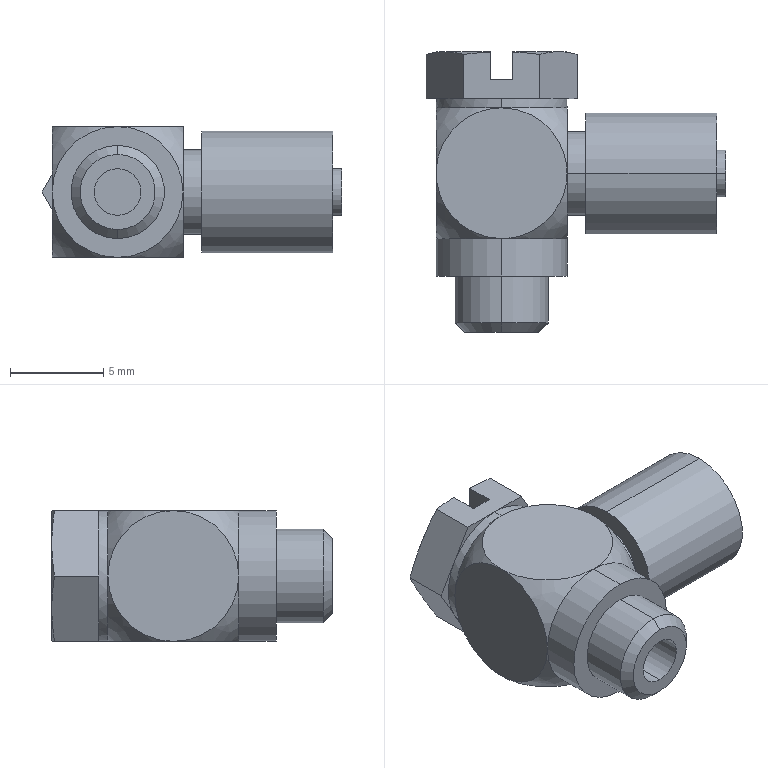Part | SolidWorks | features BaseBody 1 | 1 solid | 60 faces | box 16.041 x 15 x 7 mm | volume 771.303 mm3 | plane 28 | cylinder 16 | cone 8 | spline 8 | commonest cylinder face diameters 2.5 x4 7 x4 1.8 x2 4.5 x2 5 x2 6.5 x2